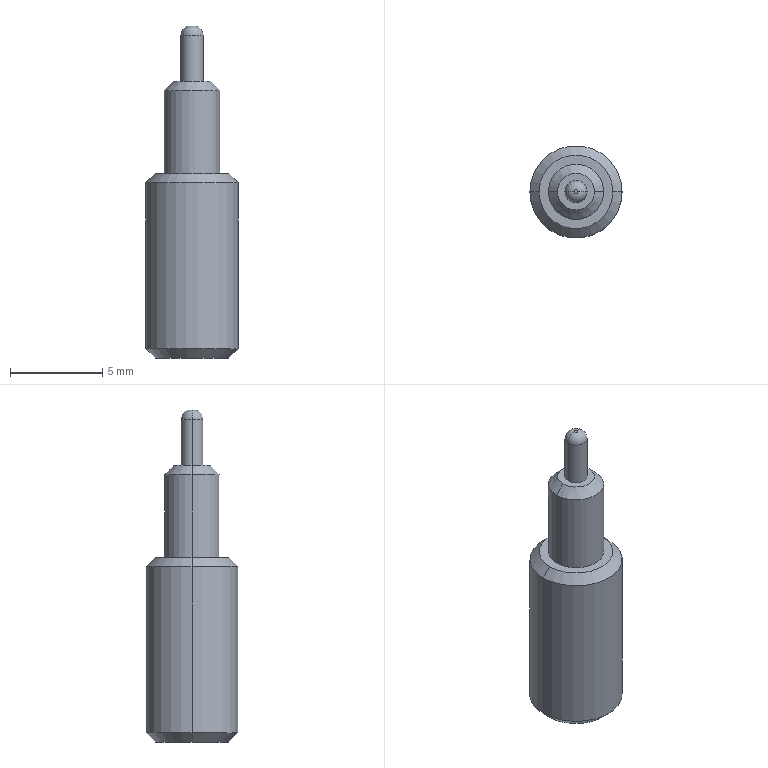Part | SolidWorks | features ICE 3, Chamfer 1, Extrusion 1, Fillet 1 | 1 solid | 21 faces | box 5 x 5 x 18 mm | volume 197.687 mm3 | cylinder 8 | cone 6 | plane 5 | torus 2 | commonest cylinder face diameters 1.2 x2 1.785 x2 3 x2 5 x2
STEP:
#1=CARTESIAN_POINT('',(-2.,0.,0.));
#2=VERTEX_POINT('',#1);
#3=CARTESIAN_POINT('',(2.,0.,0.));
#4=VERTEX_POINT('',#3);
#5=CARTESIAN_POINT('',(0.,0.,0.));
#6=DIRECTION('',(0.,0.,-1.));
#7=DIRECTION('',(1.,0.,0.));
#8=AXIS2_PLACEMENT_3D('',#5,#6,#7);
#9=CIRCLE('',#8,2.);
#10=EDGE_CURVE('',#2,#4,#9,.T.);
#11=ORIENTED_EDGE('',*,*,#10,.F.);
#12=CARTESIAN_POINT('',(-2.5,0.,0.5));
#13=VERTEX_POINT('',#12);
#14=CARTESIAN_POINT('',(-2.5,0.,0.5));
#15=DIRECTION('',(-0.7071,0.,0.7071));
#16=VECTOR('',#15,1000.);
#17=LINE('',#14,#16);
#18=EDGE_CURVE('',#2,#13,#17,.T.);
#19=ORIENTED_EDGE('',*,*,#18,.T.);
#20=CARTESIAN_POINT('',(2.5,0.,0.5));
#21=VERTEX_POINT('',#20);
#22=CARTESIAN_POINT('',(0.,0.,0.5));
#23=DIRECTION('',(0.,0.,1.));
#24=DIRECTION('',(1.,0.,0.));
#25=AXIS2_PLACEMENT_3D('',#22,#23,#24);
#26=CIRCLE('',#25,2.5);
#27=EDGE_CURVE('',#21,#13,#26,.T.);
#28=ORIENTED_EDGE('',*,*,#27,.F.);
#29=CARTESIAN_POINT('',(2.5,0.,0.5));
#30=DIRECTION('',(0.7071,0.,0.7071));
#31=VECTOR('',#30,1000.);
#32=LINE('',#29,#31);
#33=EDGE_CURVE('',#4,#21,#32,.T.);
#34=ORIENTED_EDGE('',*,*,#33,.F.);
#35=EDGE_LOOP('',(#11,#19,#28,#34));
#36=FACE_OUTER_BOUND('',#35,.T.);
#37=CARTESIAN_POINT('',(0.,0.,0.5));
#38=DIRECTION('',(0.,0.,1.));
#39=DIRECTION('',(1.,0.,0.));
#40=AXIS2_PLACEMENT_3D('',#37,#38,#39);
#41=CONICAL_SURFACE('',#40,2.5,0.7854);
#42=ADVANCED_FACE('',(#36),#41,.T.);
#43=CARTESIAN_POINT('',(2.,0.,10.));
#44=VERTEX_POINT('',#43);
#45=CARTESIAN_POINT('',(-2.,0.,10.));
#46=VERTEX_POINT('',#45);
#47=CARTESIAN_POINT('',(0.,0.,10.));
#48=DIRECTION('',(0.,0.,1.));
#49=DIRECTION('',(1.,0.,0.));
#50=AXIS2_PLACEMENT_3D('',#47,#48,#49);
#51=CIRCLE('',#50,2.);
#52=EDGE_CURVE('',#44,#46,#51,.T.);
#53=ORIENTED_EDGE('',*,*,#52,.F.);
#54=CARTESIAN_POINT('',(2.5,0.,9.5));
#55=VERTEX_POINT('',#54);
#56=CARTESIAN_POINT('',(2.,0.,10.));
#57=DIRECTION('',(0.7071,0.,-0.7071));
#58=VECTOR('',#57,1000.);
#59=LINE('',#56,#58);
#60=EDGE_CURVE('',#44,#55,#59,.T.);
#61=ORIENTED_EDGE('',*,*,#60,.T.);
#62=CARTESIAN_POINT('',(-2.5,0.,9.5));
#63=VERTEX_POINT('',#62);
#64=CARTESIAN_POINT('',(0.,0.,9.5));
#65=DIRECTION('',(0.,0.,-1.));
#66=DIRECTION('',(1.,0.,0.));
#67=AXIS2_PLACEMENT_3D('',#64,#65,#66);
#68=CIRCLE('',#67,2.5);
#69=EDGE_CURVE('',#63,#55,#68,.T.);
#70=ORIENTED_EDGE('',*,*,#69,.F.);
#71=CARTESIAN_POINT('',(-2.,0.,10.));
#72=DIRECTION('',(-0.7071,0.,-0.7071));
#73=VECTOR('',#72,1000.);
#74=LINE('',#71,#73);
#75=EDGE_CURVE('',#46,#63,#74,.T.);
#76=ORIENTED_EDGE('',*,*,#75,.F.);
#77=EDGE_LOOP('',(#53,#61,#70,#76));
#78=FACE_OUTER_BOUND('',#77,.T.);
#79=CARTESIAN_POINT('',(0.,0.,10.));
#80=DIRECTION('',(0.,0.,-1.));
#81=DIRECTION('',(-1.,0.,0.));
#82=AXIS2_PLACEMENT_3D('',#79,#80,#81);
#83=CONICAL_SURFACE('',#82,2.,0.7854);
#84=ADVANCED_FACE('',(#78),#83,.T.);
#85=CARTESIAN_POINT('',(1.,0.,15.));
#86=VERTEX_POINT('',#85);
#87=CARTESIAN_POINT('',(-1.,0.,15.));
#88=VERTEX_POINT('',#87);
#89=CARTESIAN_POINT('',(0.,0.,15.));
#90=DIRECTION('',(0.,0.,1.));
#91=DIRECTION('',(1.,0.,0.));
#92=AXIS2_PLACEMENT_3D('',#89,#90,#91);
#93=CIRCLE('',#92,1.);
#94=EDGE_CURVE('',#86,#88,#93,.T.);
#95=ORIENTED_EDGE('',*,*,#94,.F.);
#96=CARTESIAN_POINT('',(1.5,0.,14.5));
#97=VERTEX_POINT('',#96);
#98=CARTESIAN_POINT('',(1.,0.,15.));
#99=DIRECTION('',(0.7071,0.,-0.7071));
#100=VECTOR('',#99,1000.);
#101=LINE('',#98,#100);
#102=EDGE_CURVE('',#86,#97,#101,.T.);
#103=ORIENTED_EDGE('',*,*,#102,.T.);
#104=CARTESIAN_POINT('',(-1.5,0.,14.5));
#105=VERTEX_POINT('',#104);
#106=CARTESIAN_POINT('',(0.,0.,14.5));
#107=DIRECTION('',(0.,0.,-1.));
#108=DIRECTION('',(1.,0.,0.));
#109=AXIS2_PLACEMENT_3D('',#106,#107,#108);
#110=CIRCLE('',#109,1.5);
#111=EDGE_CURVE('',#105,#97,#110,.T.);
#112=ORIENTED_EDGE('',*,*,#111,.F.);
#113=CARTESIAN_POINT('',(-1.,0.,15.));
#114=DIRECTION('',(-0.7071,0.,-0.7071));
#115=VECTOR('',#114,1000.);
#116=LINE('',#113,#115);
#117=EDGE_CURVE('',#88,#105,#116,.T.);
#118=ORIENTED_EDGE('',*,*,#117,.F.);
#119=EDGE_LOOP('',(#95,#103,#112,#118));
#120=FACE_OUTER_BOUND('',#119,.T.);
#121=CARTESIAN_POINT('',(0.,0.,15.));
#122=DIRECTION('',(0.,0.,-1.));
#123=DIRECTION('',(-1.,0.,0.));
#124=AXIS2_PLACEMENT_3D('',#121,#122,#123);
#125=CONICAL_SURFACE('',#124,1.,0.7854);
#126=ADVANCED_FACE('',(#120),#125,.T.);
#127=CARTESIAN_POINT('',(0.8924,0.,13.));
#128=VERTEX_POINT('',#127);
#129=CARTESIAN_POINT('',(-0.8924,0.,13.));
#130=VERTEX_POINT('',#129);
#131=CARTESIAN_POINT('',(0.,0.,13.));
#132=DIRECTION('',(0.,0.,-1.));
#133=DIRECTION('',(-1.,0.,0.));
#134=AXIS2_PLACEMENT_3D('',#131,#132,#133);
#135=CIRCLE('',#134,0.8924);
#136=EDGE_CURVE('',#128,#130,#135,.T.);
#137=ORIENTED_EDGE('',*,*,#136,.F.);
#138=CARTESIAN_POINT('',(0.8924,0.,0.));
#139=VERTEX_POINT('',#138);
#140=CARTESIAN_POINT('',(0.8924,0.,13.));
#141=DIRECTION('',(0.,0.,-1.));
#142=VECTOR('',#141,1000.);
#143=LINE('',#140,#142);
#144=EDGE_CURVE('',#128,#139,#143,.T.);
#145=ORIENTED_EDGE('',*,*,#144,.T.);
#146=CARTESIAN_POINT('',(-0.8924,0.,0.));
#147=VERTEX_POINT('',#146);
#148=CARTESIAN_POINT('',(0.,0.,0.));
#149=DIRECTION('',(0.,0.,-1.));
#150=DIRECTION('',(-1.,0.,0.));
#151=AXIS2_PLACEMENT_3D('',#148,#149,#150);
#152=CIRCLE('',#151,0.8924);
#153=EDGE_CURVE('',#139,#147,#152,.T.);
#154=ORIENTED_EDGE('',*,*,#153,.T.);
#155=CARTESIAN_POINT('',(-0.8924,0.,13.));
#156=DIRECTION('',(0.,0.,-1.));
#157=VECTOR('',#156,1000.);
#158=LINE('',#155,#157);
#159=EDGE_CURVE('',#130,#147,#158,.T.);
#160=ORIENTED_EDGE('',*,*,#159,.F.);
#161=EDGE_LOOP('',(#137,#145,#154,#160));
#162=FACE_OUTER_BOUND('',#161,.T.);
#163=CARTESIAN_POINT('',(0.,0.,13.));
#164=DIRECTION('',(0.,0.,-1.));
#165=DIRECTION('',(-1.,0.,0.));
#166=AXIS2_PLACEMENT_3D('',#163,#164,#165);
#167=CYLINDRICAL_SURFACE('',#166,0.8924);
#168=ADVANCED_FACE('',(#162),#167,.F.);
#169=CARTESIAN_POINT('',(-0.6,0.,17.5));
#170=VERTEX_POINT('',#169);
#171=CARTESIAN_POINT('',(0.6,0.,17.5));
#172=VERTEX_POINT('',#171);
#173=CARTESIAN_POINT('',(0.,0.,17.5));
#174=DIRECTION('',(0.,0.,-1.));
#175=DIRECTION('',(1.,0.,0.));
#176=AXIS2_PLACEMENT_3D('',#173,#174,#175);
#177=CIRCLE('',#176,0.6);
#178=EDGE_CURVE('',#170,#172,#177,.T.);
#179=ORIENTED_EDGE('',*,*,#178,.F.);
#180=CARTESIAN_POINT('',(-0.1,0.,18.));
#181=VERTEX_POINT('',#180);
#182=CARTESIAN_POINT('',(-0.1,0.,17.5));
#183=DIRECTION('',(0.,1.,0.));
#184=DIRECTION('',(-1.,0.,0.));
#185=AXIS2_PLACEMENT_3D('',#182,#183,#184);
#186=CIRCLE('',#185,0.5);
#187=EDGE_CURVE('',#170,#181,#186,.T.);
#188=ORIENTED_EDGE('',*,*,#187,.T.);
#189=CARTESIAN_POINT('',(0.1,0.,18.));
#190=VERTEX_POINT('',#189);
#191=CARTESIAN_POINT('',(0.,0.,18.));
#192=DIRECTION('',(0.,0.,1.));
#193=DIRECTION('',(1.,0.,0.));
#194=AXIS2_PLACEMENT_3D('',#191,#192,#193);
#195=CIRCLE('',#194,0.1);
#196=EDGE_CURVE('',#190,#181,#195,.T.);
#197=ORIENTED_EDGE('',*,*,#196,.F.);
#198=CARTESIAN_POINT('',(0.1,0.,17.5));
#199=DIRECTION('',(0.,-1.,0.));
#200=DIRECTION('',(0.,0.,-1.));
#201=AXIS2_PLACEMENT_3D('',#198,#199,#200);
#202=CIRCLE('',#201,0.5);
#203=EDGE_CURVE('',#172,#190,#202,.T.);
#204=ORIENTED_EDGE('',*,*,#203,.F.);
#205=EDGE_LOOP('',(#179,#188,#197,#204));
#206=FACE_OUTER_BOUND('',#205,.T.);
#207=CARTESIAN_POINT('',(0.,0.,17.5));
#208=DIRECTION('',(0.,0.,1.));
#209=DIRECTION('',(1.,0.,0.));
#210=AXIS2_PLACEMENT_3D('',#207,#208,#209);
#211=TOROIDAL_SURFACE('',#210,0.1,0.5);
#212=ADVANCED_FACE('',(#206),#211,.T.);
#213=ORIENTED_EDGE('',*,*,#178,.T.);
#214=CARTESIAN_POINT('',(0.6,0.,15.));
#215=VERTEX_POINT('',#214);
#216=CARTESIAN_POINT('',(0.6,0.,18.));
#217=DIRECTION('',(0.,0.,-1.));
#218=VECTOR('',#217,1000.);
#219=LINE('',#216,#218);
#220=EDGE_CURVE('',#172,#215,#219,.T.);
#221=ORIENTED_EDGE('',*,*,#220,.T.);
#222=CARTESIAN_POINT('',(-0.6,0.,15.));
#223=VERTEX_POINT('',#222);
#224=CARTESIAN_POINT('',(0.,0.,15.));
#225=DIRECTION('',(0.,0.,1.));
#226=DIRECTION('',(1.,0.,0.));
#227=AXIS2_PLACEMENT_3D('',#224,#225,#226);
#228=CIRCLE('',#227,0.6);
#229=EDGE_CURVE('',#215,#223,#228,.T.);
#230=ORIENTED_EDGE('',*,*,#229,.T.);
#231=CARTESIAN_POINT('',(-0.6,0.,18.));
#232=DIRECTION('',(0.,0.,-1.));
#233=VECTOR('',#232,1000.);
#234=LINE('',#231,#233);
#235=EDGE_CURVE('',#170,#223,#234,.T.);
#236=ORIENTED_EDGE('',*,*,#235,.F.);
#237=EDGE_LOOP('',(#213,#221,#230,#236));
#238=FACE_OUTER_BOUND('',#237,.T.);
#239=CARTESIAN_POINT('',(0.,0.,18.));
#240=DIRECTION('',(0.,0.,-1.));
#241=DIRECTION('',(-1.,0.,0.));
#242=AXIS2_PLACEMENT_3D('',#239,#240,#241);
#243=CYLINDRICAL_SURFACE('',#242,0.6);
#244=ADVANCED_FACE('',(#238),#243,.T.);
#245=ORIENTED_EDGE('',*,*,#111,.T.);
#246=CARTESIAN_POINT('',(1.5,0.,10.));
#247=VERTEX_POINT('',#246);
#248=CARTESIAN_POINT('',(1.5,0.,15.));
#249=DIRECTION('',(0.,0.,-1.));
#250=VECTOR('',#249,1000.);
#251=LINE('',#248,#250);
#252=EDGE_CURVE('',#97,#247,#251,.T.);
#253=ORIENTED_EDGE('',*,*,#252,.T.);
#254=CARTESIAN_POINT('',(-1.5,0.,10.));
#255=VERTEX_POINT('',#254);
#256=CARTESIAN_POINT('',(0.,0.,10.));
#257=DIRECTION('',(0.,0.,1.));
#258=DIRECTION('',(1.,0.,0.));
#259=AXIS2_PLACEMENT_3D('',#256,#257,#258);
#260=CIRCLE('',#259,1.5);
#261=EDGE_CURVE('',#247,#255,#260,.T.);
#262=ORIENTED_EDGE('',*,*,#261,.T.);
#263=CARTESIAN_POINT('',(-1.5,0.,15.));
#264=DIRECTION('',(0.,0.,-1.));
#265=VECTOR('',#264,1000.);
#266=LINE('',#263,#265);
#267=EDGE_CURVE('',#105,#255,#266,.T.);
#268=ORIENTED_EDGE('',*,*,#267,.F.);
#269=EDGE_LOOP('',(#245,#253,#262,#268));
#270=FACE_OUTER_BOUND('',#269,.T.);
#271=CARTESIAN_POINT('',(0.,0.,15.));
#272=DIRECTION('',(0.,0.,-1.));
#273=DIRECTION('',(-1.,0.,0.));
#274=AXIS2_PLACEMENT_3D('',#271,#272,#273);
#275=CYLINDRICAL_SURFACE('',#274,1.5);
#276=ADVANCED_FACE('',(#270),#275,.T.);
#277=ORIENTED_EDGE('',*,*,#69,.T.);
#278=CARTESIAN_POINT('',(2.5,0.,10.));
#279=DIRECTION('',(0.,0.,-1.));
#280=VECTOR('',#279,1000.);
#281=LINE('',#278,#280);
#282=EDGE_CURVE('',#55,#21,#281,.T.);
#283=ORIENTED_EDGE('',*,*,#282,.T.);
#284=ORIENTED_EDGE('',*,*,#27,.T.);
#285=CARTESIAN_POINT('',(-2.5,0.,10.));
#286=DIRECTION('',(0.,0.,-1.));
#287=VECTOR('',#286,1000.);
#288=LINE('',#285,#287);
#289=EDGE_CURVE('',#63,#13,#288,.T.);
#290=ORIENTED_EDGE('',*,*,#289,.F.);
#291=EDGE_LOOP('',(#277,#283,#284,#290));
#292=FACE_OUTER_BOUND('',#291,.T.);
#293=CARTESIAN_POINT('',(0.,0.,10.));
#294=DIRECTION('',(0.,0.,-1.));
#295=DIRECTION('',(-1.,0.,0.));
#296=AXIS2_PLACEMENT_3D('',#293,#294,#295);
#297=CYLINDRICAL_SURFACE('',#296,2.5);
#298=ADVANCED_FACE('',(#292),#297,.T.);
#299=ORIENTED_EDGE('',*,*,#282,.F.);
#300=CARTESIAN_POINT('',(0.,0.,9.5));
#301=DIRECTION('',(0.,0.,-1.));
#302=DIRECTION('',(1.,0.,0.));
#303=AXIS2_PLACEMENT_3D('',#300,#301,#302);
#304=CIRCLE('',#303,2.5);
#305=EDGE_CURVE('',#55,#63,#304,.T.);
#306=ORIENTED_EDGE('',*,*,#305,.T.);
#307=ORIENTED_EDGE('',*,*,#289,.T.);
#308=CARTESIAN_POINT('',(0.,0.,0.5));
#309=DIRECTION('',(0.,0.,1.));
#310=DIRECTION('',(1.,0.,0.));
#311=AXIS2_PLACEMENT_3D('',#308,#309,#310);
#312=CIRCLE('',#311,2.5);
#313=EDGE_CURVE('',#13,#21,#312,.T.);
#314=ORIENTED_EDGE('',*,*,#313,.T.);
#315=EDGE_LOOP('',(#299,#306,#307,#314));
#316=FACE_OUTER_BOUND('',#315,.T.);
#317=CARTESIAN_POINT('',(0.,0.,10.));
#318=DIRECTION('',(0.,0.,-1.));
#319=DIRECTION('',(-1.,0.,0.));
#320=AXIS2_PLACEMENT_3D('',#317,#318,#319);
#321=CYLINDRICAL_SURFACE('',#320,2.5);
#322=ADVANCED_FACE('',(#316),#321,.T.);
#323=CARTESIAN_POINT('',(0.,0.,10.));
#324=DIRECTION('',(0.,0.,1.));
#325=DIRECTION('',(1.,0.,0.));
#326=AXIS2_PLACEMENT_3D('',#323,#324,#325);
#327=CIRCLE('',#326,2.);
#328=EDGE_CURVE('',#46,#44,#327,.T.);
#329=ORIENTED_EDGE('',*,*,#328,.T.);
#330=ORIENTED_EDGE('',*,*,#52,.T.);
#331=EDGE_LOOP('',(#329,#330));
#332=FACE_OUTER_BOUND('',#331,.T.);
#333=CARTESIAN_POINT('',(0.,0.,10.));
#334=DIRECTION('',(0.,0.,1.));
#335=DIRECTION('',(1.,0.,0.));
#336=AXIS2_PLACEMENT_3D('',#333,#334,#335);
#337=CIRCLE('',#336,1.5);
#338=EDGE_CURVE('',#255,#247,#337,.T.);
#339=ORIENTED_EDGE('',*,*,#338,.F.);
#340=ORIENTED_EDGE('',*,*,#261,.F.);
#341=EDGE_LOOP('',(#339,#340));
#342=FACE_BOUND('',#341,.T.);
#343=CARTESIAN_POINT('',(0.,0.,10.));
#344=DIRECTION('',(0.,0.,1.));
#345=DIRECTION('',(1.,0.,0.));
#346=AXIS2_PLACEMENT_3D('',#343,#344,#345);
#347=PLANE('',#346);
#348=ADVANCED_FACE('',(#332,#342),#347,.T.);
#349=CARTESIAN_POINT('',(0.,0.,0.));
#350=DIRECTION('',(0.,0.,-1.));
#351=DIRECTION('',(1.,0.,0.));
#352=AXIS2_PLACEMENT_3D('',#349,#350,#351);
#353=CIRCLE('',#352,2.);
#354=EDGE_CURVE('',#4,#2,#353,.T.);
#355=ORIENTED_EDGE('',*,*,#354,.T.);
#356=ORIENTED_EDGE('',*,*,#10,.T.);
#357=EDGE_LOOP('',(#355,#356));
#358=FACE_OUTER_BOUND('',#357,.T.);
#359=CARTESIAN_POINT('',(0.,0.,0.));
#360=DIRECTION('',(0.,0.,-1.));
#361=DIRECTION('',(-1.,0.,0.));
#362=AXIS2_PLACEMENT_3D('',#359,#360,#361);
#363=CIRCLE('',#362,0.8924);
#364=EDGE_CURVE('',#147,#139,#363,.T.);
#365=ORIENTED_EDGE('',*,*,#364,.F.);
#366=ORIENTED_EDGE('',*,*,#153,.F.);
#367=EDGE_LOOP('',(#365,#366));
#368=FACE_BOUND('',#367,.T.);
#369=CARTESIAN_POINT('',(0.,0.,0.));
#370=DIRECTION('',(0.,0.,1.));
#371=DIRECTION('',(1.,0.,0.));
#372=AXIS2_PLACEMENT_3D('',#369,#370,#371);
#373=PLANE('',#372);
#374=ADVANCED_FACE('',(#358,#368),#373,.F.);
#375=ORIENTED_EDGE('',*,*,#252,.F.);
#376=CARTESIAN_POINT('',(0.,0.,14.5));
#377=DIRECTION('',(0.,0.,-1.));
#378=DIRECTION('',(1.,0.,0.));
#379=AXIS2_PLACEMENT_3D('',#376,#377,#378);
#380=CIRCLE('',#379,1.5);
#381=EDGE_CURVE('',#97,#105,#380,.T.);
#382=ORIENTED_EDGE('',*,*,#381,.T.);
#383=ORIENTED_EDGE('',*,*,#267,.T.);
#384=ORIENTED_EDGE('',*,*,#338,.T.);
#385=EDGE_LOOP('',(#375,#382,#383,#384));
#386=FACE_OUTER_BOUND('',#385,.T.);
#387=CARTESIAN_POINT('',(0.,0.,15.));
#388=DIRECTION('',(0.,0.,-1.));
#389=DIRECTION('',(-1.,0.,0.));
#390=AXIS2_PLACEMENT_3D('',#387,#388,#389);
#391=CYLINDRICAL_SURFACE('',#390,1.5);
#392=ADVANCED_FACE('',(#386),#391,.T.);
#393=CARTESIAN_POINT('',(0.,0.,15.));
#394=DIRECTION('',(0.,0.,1.));
#395=DIRECTION('',(1.,0.,0.));
#396=AXIS2_PLACEMENT_3D('',#393,#394,#395);
#397=CIRCLE('',#396,1.);
#398=EDGE_CURVE('',#88,#86,#397,.T.);
#399=ORIENTED_EDGE('',*,*,#398,.T.);
#400=ORIENTED_EDGE('',*,*,#94,.T.);
#401=EDGE_LOOP('',(#399,#400));
#402=FACE_OUTER_BOUND('',#401,.T.);
#403=CARTESIAN_POINT('',(0.,0.,15.));
#404=DIRECTION('',(0.,0.,1.));
#405=DIRECTION('',(1.,0.,0.));
#406=AXIS2_PLACEMENT_3D('',#403,#404,#405);
#407=CIRCLE('',#406,0.6);
#408=EDGE_CURVE('',#223,#215,#407,.T.);
#409=ORIENTED_EDGE('',*,*,#408,.F.);
#410=ORIENTED_EDGE('',*,*,#229,.F.);
#411=EDGE_LOOP('',(#409,#410));
#412=FACE_BOUND('',#411,.T.);
#413=CARTESIAN_POINT('',(0.,0.,15.));
#414=DIRECTION('',(0.,0.,1.));
#415=DIRECTION('',(1.,0.,0.));
#416=AXIS2_PLACEMENT_3D('',#413,#414,#415);
#417=PLANE('',#416);
#418=ADVANCED_FACE('',(#402,#412),#417,.T.);
#419=ORIENTED_EDGE('',*,*,#220,.F.);
#420=CARTESIAN_POINT('',(0.,0.,17.5));
#421=DIRECTION('',(0.,0.,-1.));
#422=DIRECTION('',(1.,0.,0.));
#423=AXIS2_PLACEMENT_3D('',#420,#421,#422);
#424=CIRCLE('',#423,0.6);
#425=EDGE_CURVE('',#172,#170,#424,.T.);
#426=ORIENTED_EDGE('',*,*,#425,.T.);
#427=ORIENTED_EDGE('',*,*,#235,.T.);
#428=ORIENTED_EDGE('',*,*,#408,.T.);
#429=EDGE_LOOP('',(#419,#426,#427,#428));
#430=FACE_OUTER_BOUND('',#429,.T.);
#431=CARTESIAN_POINT('',(0.,0.,18.));
#432=DIRECTION('',(0.,0.,-1.));
#433=DIRECTION('',(-1.,0.,0.));
#434=AXIS2_PLACEMENT_3D('',#431,#432,#433);
#435=CYLINDRICAL_SURFACE('',#434,0.6);
#436=ADVANCED_FACE('',(#430),#435,.T.);
#437=ORIENTED_EDGE('',*,*,#196,.T.);
#438=CARTESIAN_POINT('',(0.,0.,18.));
#439=DIRECTION('',(0.,0.,1.));
#440=DIRECTION('',(1.,0.,0.));
#441=AXIS2_PLACEMENT_3D('',#438,#439,#440);
#442=CIRCLE('',#441,0.1);
#443=EDGE_CURVE('',#181,#190,#442,.T.);
#444=ORIENTED_EDGE('',*,*,#443,.T.);
#445=EDGE_LOOP('',(#437,#444));
#446=FACE_OUTER_BOUND('',#445,.T.);
#447=CARTESIAN_POINT('',(0.,0.,18.));
#448=DIRECTION('',(0.,0.,1.));
#449=DIRECTION('',(1.,0.,0.));
#450=AXIS2_PLACEMENT_3D('',#447,#448,#449);
#451=PLANE('',#450);
#452=ADVANCED_FACE('',(#446),#451,.T.);
#453=ORIENTED_EDGE('',*,*,#187,.F.);
#454=ORIENTED_EDGE('',*,*,#425,.F.);
#455=ORIENTED_EDGE('',*,*,#203,.T.);
#456=ORIENTED_EDGE('',*,*,#443,.F.);
#457=EDGE_LOOP('',(#453,#454,#455,#456));
#458=FACE_OUTER_BOUND('',#457,.T.);
#459=CARTESIAN_POINT('',(0.,0.,17.5));
#460=DIRECTION('',(0.,0.,1.));
#461=DIRECTION('',(1.,0.,0.));
#462=AXIS2_PLACEMENT_3D('',#459,#460,#461);
#463=TOROIDAL_SURFACE('',#462,0.1,0.5);
#464=ADVANCED_FACE('',(#458),#463,.T.);
#465=ORIENTED_EDGE('',*,*,#144,.F.);
#466=CARTESIAN_POINT('',(0.,0.,13.));
#467=DIRECTION('',(0.,0.,-1.));
#468=DIRECTION('',(-1.,0.,0.));
#469=AXIS2_PLACEMENT_3D('',#466,#467,#468);
#470=CIRCLE('',#469,0.8924);
#471=EDGE_CURVE('',#130,#128,#470,.T.);
#472=ORIENTED_EDGE('',*,*,#471,.F.);
#473=ORIENTED_EDGE('',*,*,#159,.T.);
#474=ORIENTED_EDGE('',*,*,#364,.T.);
#475=EDGE_LOOP('',(#465,#472,#473,#474));
#476=FACE_OUTER_BOUND('',#475,.T.);
#477=CARTESIAN_POINT('',(0.,0.,13.));
#478=DIRECTION('',(0.,0.,-1.));
#479=DIRECTION('',(-1.,0.,0.));
#480=AXIS2_PLACEMENT_3D('',#477,#478,#479);
#481=CYLINDRICAL_SURFACE('',#480,0.8924);
#482=ADVANCED_FACE('',(#476),#481,.F.);
#483=ORIENTED_EDGE('',*,*,#471,.T.);
#484=ORIENTED_EDGE('',*,*,#136,.T.);
#485=EDGE_LOOP('',(#483,#484));
#486=FACE_OUTER_BOUND('',#485,.T.);
#487=CARTESIAN_POINT('',(0.,0.,13.));
#488=DIRECTION('',(0.,0.,-1.));
#489=DIRECTION('',(-1.,0.,0.));
#490=AXIS2_PLACEMENT_3D('',#487,#488,#489);
#491=PLANE('',#490);
#492=ADVANCED_FACE('',(#486),#491,.T.);
#493=ORIENTED_EDGE('',*,*,#102,.F.);
#494=ORIENTED_EDGE('',*,*,#398,.F.);
#495=ORIENTED_EDGE('',*,*,#117,.T.);
#496=ORIENTED_EDGE('',*,*,#381,.F.);
#497=EDGE_LOOP('',(#493,#494,#495,#496));
#498=FACE_OUTER_BOUND('',#497,.T.);
#499=CARTESIAN_POINT('',(0.,0.,15.));
#500=DIRECTION('',(0.,0.,-1.));
#501=DIRECTION('',(-1.,0.,0.));
#502=AXIS2_PLACEMENT_3D('',#499,#500,#501);
#503=CONICAL_SURFACE('',#502,1.,0.7854);
#504=ADVANCED_FACE('',(#498),#503,.T.);
#505=ORIENTED_EDGE('',*,*,#60,.F.);
#506=ORIENTED_EDGE('',*,*,#328,.F.);
#507=ORIENTED_EDGE('',*,*,#75,.T.);
#508=ORIENTED_EDGE('',*,*,#305,.F.);
#509=EDGE_LOOP('',(#505,#506,#507,#508));
#510=FACE_OUTER_BOUND('',#509,.T.);
#511=CARTESIAN_POINT('',(0.,0.,10.));
#512=DIRECTION('',(0.,0.,-1.));
#513=DIRECTION('',(-1.,0.,0.));
#514=AXIS2_PLACEMENT_3D('',#511,#512,#513);
#515=CONICAL_SURFACE('',#514,2.,0.7854);
#516=ADVANCED_FACE('',(#510),#515,.T.);
#517=ORIENTED_EDGE('',*,*,#18,.F.);
#518=ORIENTED_EDGE('',*,*,#354,.F.);
#519=ORIENTED_EDGE('',*,*,#33,.T.);
#520=ORIENTED_EDGE('',*,*,#313,.F.);
#521=EDGE_LOOP('',(#517,#518,#519,#520));
#522=FACE_OUTER_BOUND('',#521,.T.);
#523=CARTESIAN_POINT('',(0.,0.,0.5));
#524=DIRECTION('',(0.,0.,1.));
#525=DIRECTION('',(1.,0.,0.));
#526=AXIS2_PLACEMENT_3D('',#523,#524,#525);
#527=CONICAL_SURFACE('',#526,2.5,0.7854);
#528=ADVANCED_FACE('',(#522),#527,.T.);
#529=CLOSED_SHELL('',(#42,#84,#126,#168,#212,#244,#276,#298,#322,#348,#374,#392,#418,#436,#452,#464,#482,#492,#504,#516,#528));
#530=MANIFOLD_SOLID_BREP('',#529);
#531=CARTESIAN_POINT('',(0.,0.,0.));
#532=DIRECTION('',(0.,0.,1.));
#533=DIRECTION('',(1.,0.,0.));
#534=AXIS2_PLACEMENT_3D('',#531,#532,#533);
#535=(LENGTH_UNIT()NAMED_UNIT(*)SI_UNIT(.MILLI.,.METRE.));
#536=UNCERTAINTY_MEASURE_WITH_UNIT(LENGTH_MEASURE(0.00001),#535,'','');
#537=(NAMED_UNIT(*)PLANE_ANGLE_UNIT()SI_UNIT($,.RADIAN.));
#538=(NAMED_UNIT(*)SI_UNIT($,.STERADIAN.)SOLID_ANGLE_UNIT());
#539=(GEOMETRIC_REPRESENTATION_CONTEXT(3)GLOBAL_UNCERTAINTY_ASSIGNED_CONTEXT((#536))GLOBAL_UNIT_ASSIGNED_CONTEXT((#535,#537,#538))REPRESENTATION_CONTEXT('',''));
#540=ADVANCED_BREP_SHAPE_REPRESENTATION('',(#530,#534),#539);